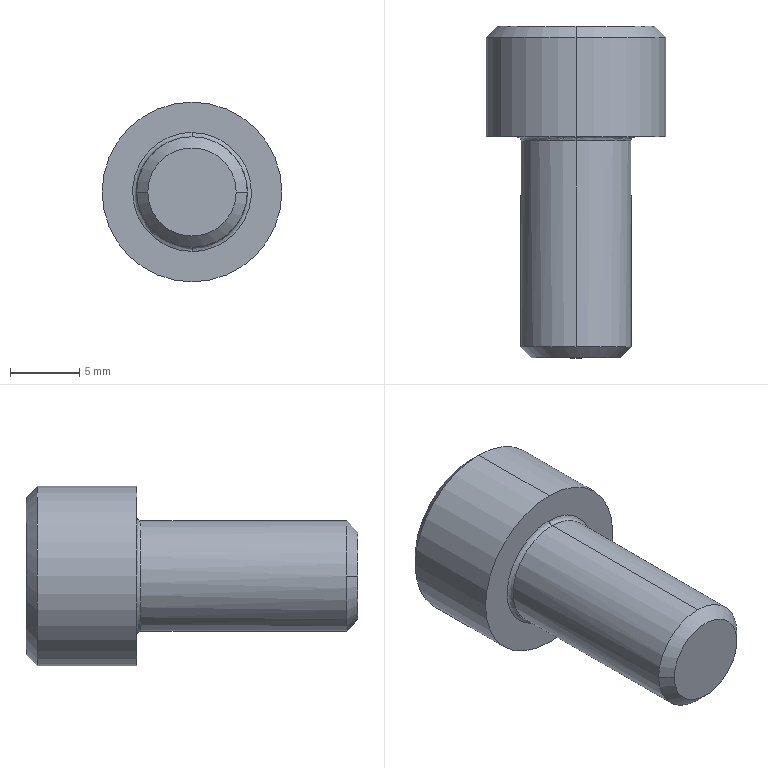Part | STEP file | 1 solid | 20 faces | box 13 x 24 x 13 mm | volume 1660 mm3 | plane 10 | cone 4 | cylinder 4 | spline 2 | commonest cylinder face diameters 8 x2 13 x2